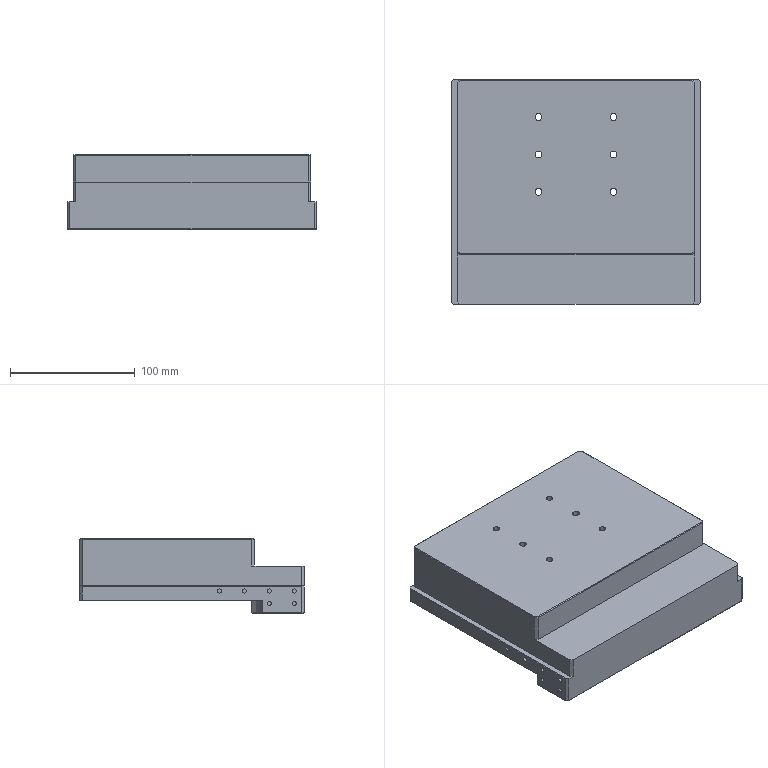Part | 1 solid | 226 faces | box 200 x 180 x 60 mm | volume 1606314 mm3 | cylinder 113 | plane 108 | cone 5 | commonest cylinder face diameters 4.2 x36 3.3 x32 2.5 x12 5.5 x12 10 x12 44 x5